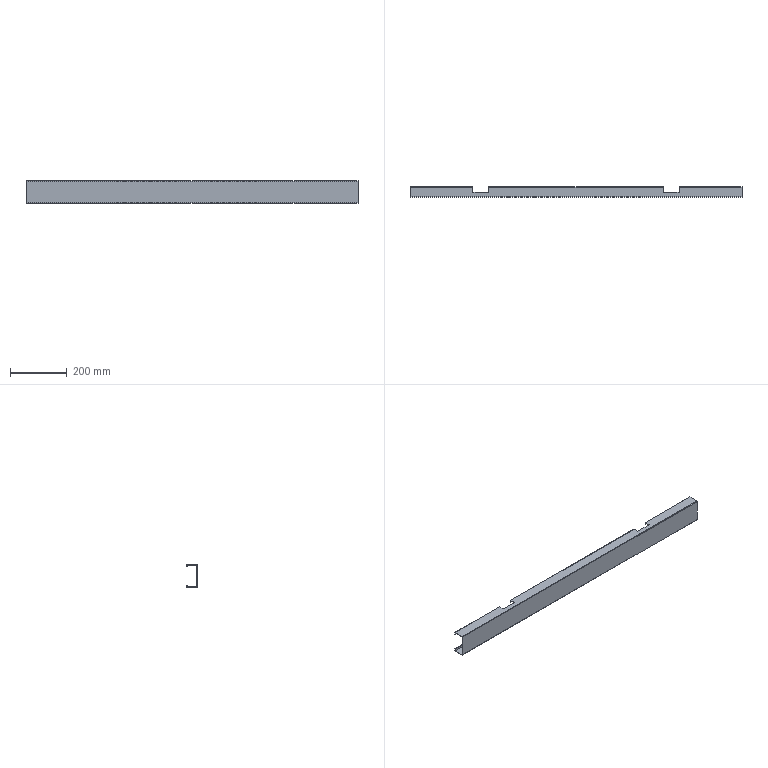Part | SolidWorks | features FlatPattern 1, ICE 1, SMBaseFlange 1, SheetMetal 1 | 1 solid | 86 faces | box 1169 x 38 x 80 mm | volume 279454 mm3 | plane 70 | cylinder 16 | commonest cylinder face diameters 0.4 x8 3.4 x8